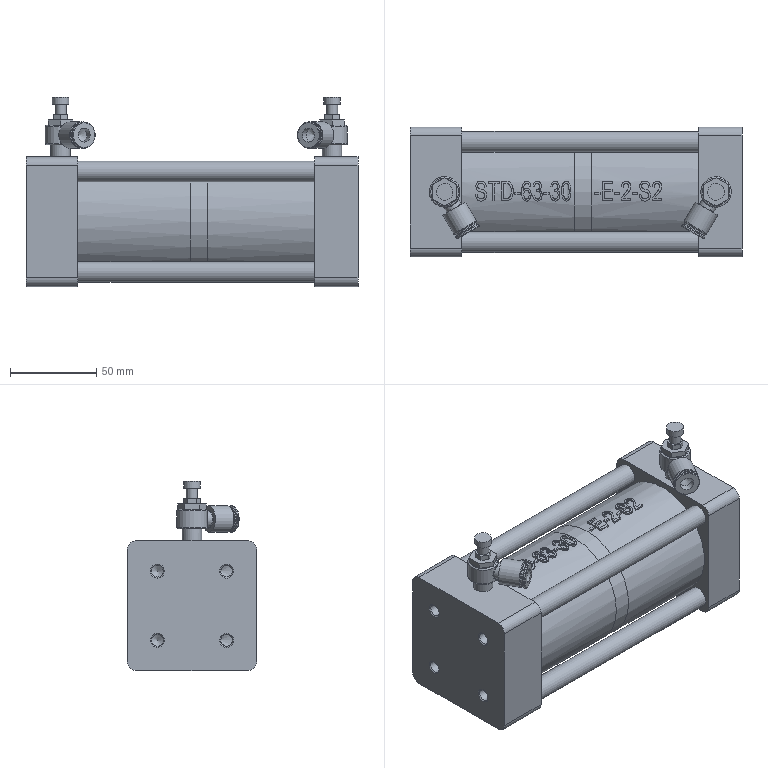Part | STEP file | Tube necking machine_id590_x_t | 1 solid | 244 faces | box 192 x 75 x 109.4 mm | volume 879096 mm3 | plane 114 | cylinder 56 | spline 48 | torus 16 | cone 10 | commonest cylinder face diameters 70 x16 10 x8 68 x6 6.8 x4 12 x4 15.2 x4